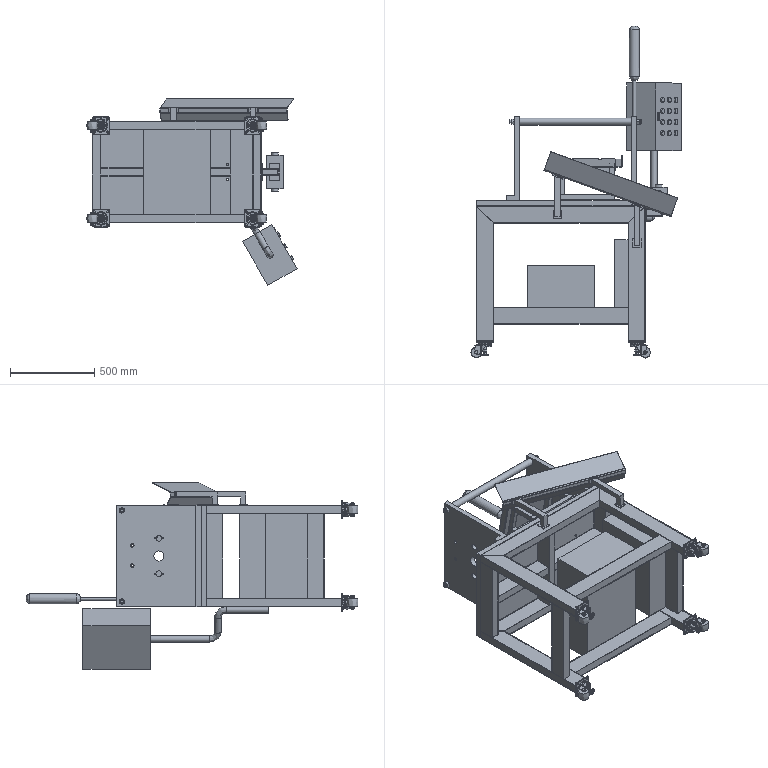Part | NX | features main frame_Default_As Machined_ 25, guide rail pipe2_Default_As Machined_ 20, Panel 16, CMAS65-F 12, output director 8, push bottom 6, Hexagon Nut ISO - 4034 - M20 - N_Hexagon Nut ISO - 4034 - M20 - N 2, Hydrolic power unit 2, information lamp 2, main panel 2 | 121 solids | 1407 faces | box 1246 x 1967 x 1107 mm | volume 170914110 mm3 | plane 891 | cylinder 315 | cone 158 | spline 43 | commonest cylinder face diameters 10 x47 20 x46 11 x32 30 x28 22 x26 16 x20